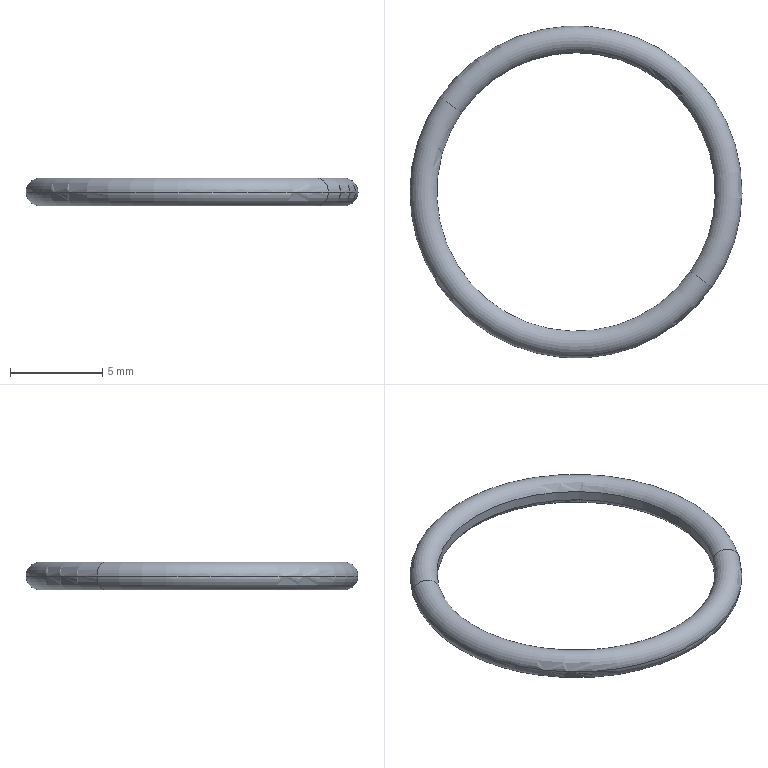Part | SolidWorks | features BaseBody 1 | 1 solid | 7 faces | box 18 x 18 x 1.5 mm | volume 90.747 mm3 | torus 4 | cylinder 3 | commonest cylinder face diameters 15.1 x3
STEP:
#1=CARTESIAN_POINT('',(97.346,-206.367,4.981));
#2=VERTEX_POINT('',#1);
#3=CARTESIAN_POINT('',(84.954,-197.739,4.981));
#4=VERTEX_POINT('',#3);
#5=CARTESIAN_POINT('',(91.15,-202.053,4.981));
#6=DIRECTION('',(0.,0.,-1.));
#7=DIRECTION('',(0.8207,-0.5714,0.));
#8=AXIS2_PLACEMENT_3D('',#5,#6,#7);
#9=CIRCLE('',#8,7.55);
#10=EDGE_CURVE('',#2,#4,#9,.T.);
#11=ORIENTED_EDGE('',*,*,#10,.T.);
#12=CARTESIAN_POINT('',(84.954,-197.739,5.519));
#13=VERTEX_POINT('',#12);
#14=CARTESIAN_POINT('',(84.954,-197.739,5.519));
#15=DIRECTION('',(0.,0.,-1.));
#16=VECTOR('',#15,1000.);
#17=LINE('',#14,#16);
#18=EDGE_CURVE('',#13,#4,#17,.T.);
#19=ORIENTED_EDGE('',*,*,#18,.F.);
#20=CARTESIAN_POINT('',(97.346,-206.367,5.519));
#21=VERTEX_POINT('',#20);
#22=CARTESIAN_POINT('',(91.15,-202.053,5.519));
#23=DIRECTION('',(0.,0.,1.));
#24=DIRECTION('',(-0.8207,0.5714,0.));
#25=AXIS2_PLACEMENT_3D('',#22,#23,#24);
#26=CIRCLE('',#25,7.55);
#27=EDGE_CURVE('',#13,#21,#26,.T.);
#28=ORIENTED_EDGE('',*,*,#27,.T.);
#29=CARTESIAN_POINT('',(97.346,-206.367,4.981));
#30=DIRECTION('',(0.,0.,1.));
#31=VECTOR('',#30,1000.);
#32=LINE('',#29,#31);
#33=EDGE_CURVE('',#2,#21,#32,.T.);
#34=ORIENTED_EDGE('',*,*,#33,.F.);
#35=EDGE_LOOP('',(#11,#19,#28,#34));
#36=FACE_OUTER_BOUND('',#35,.T.);
#37=CARTESIAN_POINT('',(91.15,-202.053,5.25));
#38=DIRECTION('',(0.,0.,-1.));
#39=DIRECTION('',(0.9993,-0.03741,0.));
#40=AXIS2_PLACEMENT_3D('',#37,#38,#39);
#41=CYLINDRICAL_SURFACE('',#40,7.55);
#42=ADVANCED_FACE('',(#36),#41,.F.);
#43=CARTESIAN_POINT('',(98.694,-202.335,5.519));
#44=VERTEX_POINT('',#43);
#45=CARTESIAN_POINT('',(98.694,-202.335,4.981));
#46=VERTEX_POINT('',#45);
#47=CARTESIAN_POINT('',(98.694,-202.335,5.25));
#48=DIRECTION('',(0.,0.,-1.));
#49=VECTOR('',#48,1000.);
#50=LINE('',#47,#49);
#51=EDGE_CURVE('',#44,#46,#50,.T.);
#52=ORIENTED_EDGE('',*,*,#51,.F.);
#53=CARTESIAN_POINT('',(91.15,-202.053,5.519));
#54=DIRECTION('',(0.,0.,1.));
#55=DIRECTION('',(0.9993,-0.03741,0.));
#56=AXIS2_PLACEMENT_3D('',#53,#54,#55);
#57=CIRCLE('',#56,7.55);
#58=EDGE_CURVE('',#44,#13,#57,.T.);
#59=ORIENTED_EDGE('',*,*,#58,.T.);
#60=ORIENTED_EDGE('',*,*,#18,.T.);
#61=CARTESIAN_POINT('',(91.15,-202.053,4.981));
#62=DIRECTION('',(0.,0.,-1.));
#63=DIRECTION('',(-0.8207,0.5714,0.));
#64=AXIS2_PLACEMENT_3D('',#61,#62,#63);
#65=CIRCLE('',#64,7.55);
#66=EDGE_CURVE('',#4,#46,#65,.T.);
#67=ORIENTED_EDGE('',*,*,#66,.T.);
#68=EDGE_LOOP('',(#52,#59,#60,#67));
#69=FACE_OUTER_BOUND('',#68,.T.);
#70=CARTESIAN_POINT('',(91.15,-202.053,5.25));
#71=DIRECTION('',(0.,0.,-1.));
#72=DIRECTION('',(0.9993,-0.03741,0.));
#73=AXIS2_PLACEMENT_3D('',#70,#71,#72);
#74=CYLINDRICAL_SURFACE('',#73,7.55);
#75=ADVANCED_FACE('',(#69),#74,.F.);
#76=CARTESIAN_POINT('',(91.15,-202.053,5.519));
#77=DIRECTION('',(0.,0.,1.));
#78=DIRECTION('',(0.9993,-0.03741,0.));
#79=AXIS2_PLACEMENT_3D('',#76,#77,#78);
#80=CIRCLE('',#79,7.55);
#81=EDGE_CURVE('',#21,#44,#80,.T.);
#82=ORIENTED_EDGE('',*,*,#81,.F.);
#83=CARTESIAN_POINT('',(98.536,-207.196,5.25));
#84=VERTEX_POINT('',#83);
#85=CARTESIAN_POINT('',(97.92,-206.767,5.25));
#86=DIRECTION('',(0.5714,0.8207,0.));
#87=DIRECTION('',(-0.766,0.5333,0.359));
#88=AXIS2_PLACEMENT_3D('',#85,#86,#87);
#89=CIRCLE('',#88,0.75);
#90=EDGE_CURVE('',#21,#84,#89,.T.);
#91=ORIENTED_EDGE('',*,*,#90,.T.);
#92=CARTESIAN_POINT('',(83.764,-196.91,5.25));
#93=VERTEX_POINT('',#92);
#94=CARTESIAN_POINT('',(91.15,-202.053,5.25));
#95=DIRECTION('',(0.,0.,-1.));
#96=DIRECTION('',(-0.8207,0.5714,0.));
#97=AXIS2_PLACEMENT_3D('',#94,#95,#96);
#98=CIRCLE('',#97,9.);
#99=EDGE_CURVE('',#93,#84,#98,.T.);
#100=ORIENTED_EDGE('',*,*,#99,.F.);
#101=CARTESIAN_POINT('',(84.379,-197.339,5.25));
#102=DIRECTION('',(-0.5714,-0.8207,0.));
#103=DIRECTION('',(0.766,-0.5333,0.359));
#104=AXIS2_PLACEMENT_3D('',#101,#102,#103);
#105=CIRCLE('',#104,0.75);
#106=EDGE_CURVE('',#13,#93,#105,.T.);
#107=ORIENTED_EDGE('',*,*,#106,.F.);
#108=ORIENTED_EDGE('',*,*,#58,.F.);
#109=EDGE_LOOP('',(#82,#91,#100,#107,#108));
#110=FACE_OUTER_BOUND('',#109,.T.);
#111=CARTESIAN_POINT('',(91.15,-202.053,5.25));
#112=DIRECTION('',(0.,0.,1.));
#113=DIRECTION('',(-0.8207,0.5714,0.));
#114=AXIS2_PLACEMENT_3D('',#111,#112,#113);
#115=TOROIDAL_SURFACE('',#114,8.25,0.75);
#116=ADVANCED_FACE('',(#110),#115,.T.);
#117=ORIENTED_EDGE('',*,*,#27,.F.);
#118=ORIENTED_EDGE('',*,*,#106,.T.);
#119=CARTESIAN_POINT('',(91.15,-202.053,5.25));
#120=DIRECTION('',(0.,0.,-1.));
#121=DIRECTION('',(0.8207,-0.5714,0.));
#122=AXIS2_PLACEMENT_3D('',#119,#120,#121);
#123=CIRCLE('',#122,9.);
#124=EDGE_CURVE('',#84,#93,#123,.T.);
#125=ORIENTED_EDGE('',*,*,#124,.F.);
#126=ORIENTED_EDGE('',*,*,#90,.F.);
#127=EDGE_LOOP('',(#117,#118,#125,#126));
#128=FACE_OUTER_BOUND('',#127,.T.);
#129=CARTESIAN_POINT('',(91.15,-202.053,5.25));
#130=DIRECTION('',(0.,0.,1.));
#131=DIRECTION('',(-0.8207,0.5714,0.));
#132=AXIS2_PLACEMENT_3D('',#129,#130,#131);
#133=TOROIDAL_SURFACE('',#132,8.25,0.75);
#134=ADVANCED_FACE('',(#128),#133,.T.);
#135=ORIENTED_EDGE('',*,*,#124,.T.);
#136=CARTESIAN_POINT('',(84.379,-197.339,5.25));
#137=DIRECTION('',(-0.5714,-0.8207,0.));
#138=DIRECTION('',(-0.8207,0.5714,0.));
#139=AXIS2_PLACEMENT_3D('',#136,#137,#138);
#140=CIRCLE('',#139,0.75);
#141=EDGE_CURVE('',#93,#4,#140,.T.);
#142=ORIENTED_EDGE('',*,*,#141,.T.);
#143=ORIENTED_EDGE('',*,*,#10,.F.);
#144=CARTESIAN_POINT('',(97.92,-206.767,5.25));
#145=DIRECTION('',(0.5714,0.8207,0.));
#146=DIRECTION('',(0.8207,-0.5714,0.));
#147=AXIS2_PLACEMENT_3D('',#144,#145,#146);
#148=CIRCLE('',#147,0.75);
#149=EDGE_CURVE('',#84,#2,#148,.T.);
#150=ORIENTED_EDGE('',*,*,#149,.F.);
#151=EDGE_LOOP('',(#135,#142,#143,#150));
#152=FACE_OUTER_BOUND('',#151,.T.);
#153=CARTESIAN_POINT('',(91.15,-202.053,5.25));
#154=DIRECTION('',(0.,0.,1.));
#155=DIRECTION('',(-0.8207,0.5714,0.));
#156=AXIS2_PLACEMENT_3D('',#153,#154,#155);
#157=TOROIDAL_SURFACE('',#156,8.25,0.75);
#158=ADVANCED_FACE('',(#152),#157,.T.);
#159=ORIENTED_EDGE('',*,*,#66,.F.);
#160=ORIENTED_EDGE('',*,*,#141,.F.);
#161=ORIENTED_EDGE('',*,*,#99,.T.);
#162=ORIENTED_EDGE('',*,*,#149,.T.);
#163=CARTESIAN_POINT('',(91.15,-202.053,4.981));
#164=DIRECTION('',(0.,0.,-1.));
#165=DIRECTION('',(-0.8207,0.5714,0.));
#166=AXIS2_PLACEMENT_3D('',#163,#164,#165);
#167=CIRCLE('',#166,7.55);
#168=EDGE_CURVE('',#46,#2,#167,.T.);
#169=ORIENTED_EDGE('',*,*,#168,.F.);
#170=EDGE_LOOP('',(#159,#160,#161,#162,#169));
#171=FACE_OUTER_BOUND('',#170,.T.);
#172=CARTESIAN_POINT('',(91.15,-202.053,5.25));
#173=DIRECTION('',(0.,0.,1.));
#174=DIRECTION('',(-0.8207,0.5714,0.));
#175=AXIS2_PLACEMENT_3D('',#172,#173,#174);
#176=TOROIDAL_SURFACE('',#175,8.25,0.75);
#177=ADVANCED_FACE('',(#171),#176,.T.);
#178=ORIENTED_EDGE('',*,*,#81,.T.);
#179=ORIENTED_EDGE('',*,*,#51,.T.);
#180=ORIENTED_EDGE('',*,*,#168,.T.);
#181=ORIENTED_EDGE('',*,*,#33,.T.);
#182=EDGE_LOOP('',(#178,#179,#180,#181));
#183=FACE_OUTER_BOUND('',#182,.T.);
#184=CARTESIAN_POINT('',(91.15,-202.053,5.25));
#185=DIRECTION('',(0.,0.,-1.));
#186=DIRECTION('',(0.9993,-0.03741,0.));
#187=AXIS2_PLACEMENT_3D('',#184,#185,#186);
#188=CYLINDRICAL_SURFACE('',#187,7.55);
#189=ADVANCED_FACE('',(#183),#188,.F.);
#190=CLOSED_SHELL('',(#42,#75,#116,#134,#158,#177,#189));
#191=MANIFOLD_SOLID_BREP('',#190);
#192=CARTESIAN_POINT('',(0.,0.,0.));
#193=DIRECTION('',(0.,0.,1.));
#194=DIRECTION('',(1.,0.,0.));
#195=AXIS2_PLACEMENT_3D('',#192,#193,#194);
#196=(LENGTH_UNIT()NAMED_UNIT(*)SI_UNIT(.MILLI.,.METRE.));
#197=UNCERTAINTY_MEASURE_WITH_UNIT(LENGTH_MEASURE(0.00001),#196,'','');
#198=(NAMED_UNIT(*)PLANE_ANGLE_UNIT()SI_UNIT($,.RADIAN.));
#199=(NAMED_UNIT(*)SI_UNIT($,.STERADIAN.)SOLID_ANGLE_UNIT());
#200=(GEOMETRIC_REPRESENTATION_CONTEXT(3)GLOBAL_UNCERTAINTY_ASSIGNED_CONTEXT((#197))GLOBAL_UNIT_ASSIGNED_CONTEXT((#196,#198,#199))REPRESENTATION_CONTEXT('',''));
#201=ADVANCED_BREP_SHAPE_REPRESENTATION('',(#191,#195),#200);